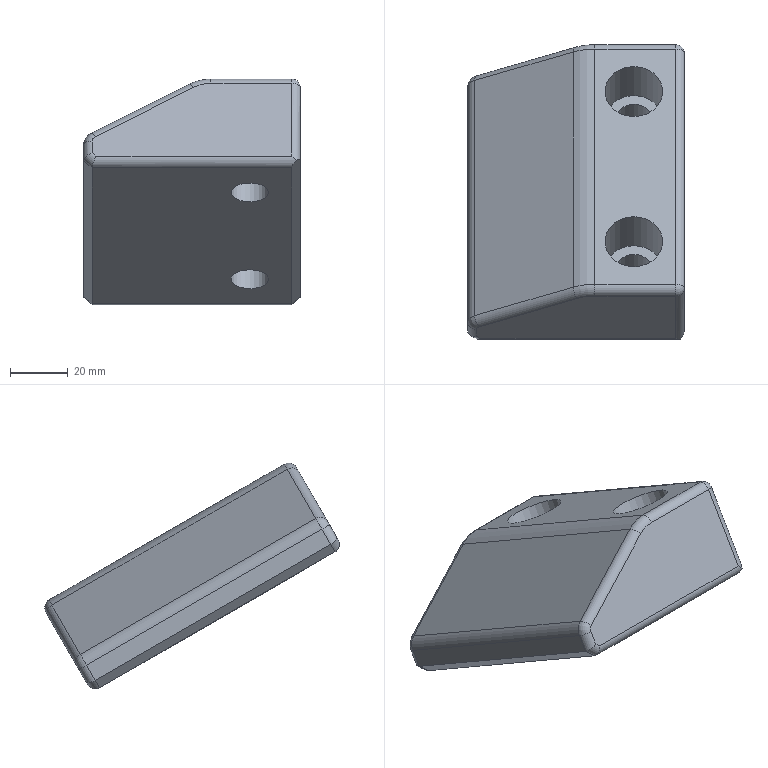Part | NX | features MAIN_BODY 2 | 1 solid | 37 faces | box 75 x 101.906 x 78.115 mm | volume 197655 mm3 | cylinder 20 | plane 11 | torus 4 | sphere 2 | commonest cylinder face diameters 6 x14 13 x2 20 x2 10 x1 30 x1
STEP:
#1=CARTESIAN_POINT('',(342.,445.056,-333.141));
#2=VERTEX_POINT('',#1);
#3=CARTESIAN_POINT('',(342.,363.649,-286.141));
#4=VERTEX_POINT('',#3);
#5=CARTESIAN_POINT('',(342.,361.051,-284.641));
#6=DIRECTION('',(0.,0.866,-0.5));
#7=VECTOR('',#6,1000.);
#8=LINE('',#5,#7);
#9=EDGE_CURVE('',#2,#4,#8,.F.);
#10=ORIENTED_EDGE('',*,*,#9,.F.);
#11=CARTESIAN_POINT('',(342.,442.046,-338.354));
#12=VERTEX_POINT('',#11);
#13=CARTESIAN_POINT('',(342.,445.056,-333.141));
#14=DIRECTION('',(0.,-0.5,-0.866));
#15=VECTOR('',#14,1000.);
#16=LINE('',#13,#15);
#17=EDGE_CURVE('',#12,#2,#16,.F.);
#18=ORIENTED_EDGE('',*,*,#17,.F.);
#19=CARTESIAN_POINT('',(342.,360.64,-291.354));
#20=VERTEX_POINT('',#19);
#21=CARTESIAN_POINT('',(342.,487.945,-364.854));
#22=DIRECTION('',(0.,0.866,-0.5));
#23=VECTOR('',#22,1000.);
#24=LINE('',#21,#23);
#25=EDGE_CURVE('',#20,#12,#24,.T.);
#26=ORIENTED_EDGE('',*,*,#25,.F.);
#27=CARTESIAN_POINT('',(342.,355.14,-300.88));
#28=DIRECTION('',(0.,-0.5,-0.866));
#29=VECTOR('',#28,1000.);
#30=LINE('',#27,#29);
#31=EDGE_CURVE('',#4,#20,#30,.T.);
#32=ORIENTED_EDGE('',*,*,#31,.F.);
#33=EDGE_LOOP('',(#10,#18,#26,#32));
#34=FACE_BOUND('',#33,.T.);
#35=CARTESIAN_POINT('',(342.,692.024,-495.38));
#36=DIRECTION('',(1.,0.,0.));
#37=DIRECTION('',(0.,0.342,-0.9397));
#38=AXIS2_PLACEMENT_3D('',#35,#36,#37);
#39=PLANE('',#38);
#40=ADVANCED_FACE('',(#34),#39,.F.);
#41=CARTESIAN_POINT('',(399.5,400.022,-277.141));
#42=VERTEX_POINT('',#41);
#43=CARTESIAN_POINT('',(399.5,391.362,-272.141));
#44=DIRECTION('',(0.,0.5,0.866));
#45=DIRECTION('',(0.,0.866,-0.5));
#46=AXIS2_PLACEMENT_3D('',#43,#44,#45);
#47=CIRCLE('',#46,10.);
#48=EDGE_CURVE('',#42,#42,#47,.T.);
#49=ORIENTED_EDGE('',*,*,#48,.F.);
#50=EDGE_LOOP('',(#49));
#51=FACE_BOUND('',#50,.T.);
#52=CARTESIAN_POINT('',(399.5,451.984,-307.141));
#53=VERTEX_POINT('',#52);
#54=CARTESIAN_POINT('',(399.5,443.324,-302.141));
#55=DIRECTION('',(0.,0.5,0.866));
#56=DIRECTION('',(0.,0.866,-0.5));
#57=AXIS2_PLACEMENT_3D('',#54,#55,#56);
#58=CIRCLE('',#57,10.);
#59=EDGE_CURVE('',#53,#53,#58,.T.);
#60=ORIENTED_EDGE('',*,*,#59,.F.);
#61=EDGE_LOOP('',(#60));
#62=FACE_BOUND('',#61,.T.);
#63=CARTESIAN_POINT('',(414.,458.046,-310.641));
#64=VERTEX_POINT('',#63);
#65=CARTESIAN_POINT('',(414.,376.64,-263.641));
#66=VERTEX_POINT('',#65);
#67=CARTESIAN_POINT('',(414.,629.519,-409.641));
#68=DIRECTION('',(0.,-0.866,0.5));
#69=VECTOR('',#68,1000.);
#70=LINE('',#67,#69);
#71=EDGE_CURVE('',#64,#66,#70,.T.);
#72=ORIENTED_EDGE('',*,*,#71,.F.);
#73=CARTESIAN_POINT('',(386.019,458.046,-310.641));
#74=VERTEX_POINT('',#73);
#75=CARTESIAN_POINT('',(467.,458.046,-310.641));
#76=DIRECTION('',(1.,0.,0.));
#77=VECTOR('',#76,1000.);
#78=LINE('',#75,#77);
#79=EDGE_CURVE('',#74,#64,#78,.T.);
#80=ORIENTED_EDGE('',*,*,#79,.F.);
#81=CARTESIAN_POINT('',(386.019,376.64,-263.641));
#82=VERTEX_POINT('',#81);
#83=CARTESIAN_POINT('',(386.019,629.519,-409.641));
#84=DIRECTION('',(0.,-0.866,0.5));
#85=VECTOR('',#84,1000.);
#86=LINE('',#83,#85);
#87=EDGE_CURVE('',#82,#74,#86,.F.);
#88=ORIENTED_EDGE('',*,*,#87,.F.);
#89=CARTESIAN_POINT('',(386.019,376.64,-263.641));
#90=DIRECTION('',(-1.,0.,0.));
#91=VECTOR('',#90,1000.);
#92=LINE('',#89,#91);
#93=EDGE_CURVE('',#66,#82,#92,.T.);
#94=ORIENTED_EDGE('',*,*,#93,.F.);
#95=EDGE_LOOP('',(#72,#80,#88,#94));
#96=FACE_BOUND('',#95,.T.);
#97=CARTESIAN_POINT('',(467.,629.519,-409.641));
#98=DIRECTION('',(0.,0.5,0.866));
#99=DIRECTION('',(0.,-0.866,0.5));
#100=AXIS2_PLACEMENT_3D('',#97,#98,#99);
#101=PLANE('',#100);
#102=ADVANCED_FACE('',(#51,#62,#96),#101,.T.);
#103=CARTESIAN_POINT('',(345.,445.265,-338.778));
#104=VERTEX_POINT('',#103);
#105=CARTESIAN_POINT('',(346.243,444.644,-339.854));
#106=VERTEX_POINT('',#105);
#107=CARTESIAN_POINT('',(315.621,459.955,-313.335));
#108=DIRECTION('',(0.7071,-0.3536,-0.6124));
#109=VECTOR('',#108,1000.);
#110=LINE('',#107,#109);
#111=EDGE_CURVE('',#104,#106,#110,.T.);
#112=ORIENTED_EDGE('',*,*,#111,.F.);
#113=CARTESIAN_POINT('',(345.,447.654,-334.641));
#114=VERTEX_POINT('',#113);
#115=CARTESIAN_POINT('',(345.,444.644,-339.854));
#116=DIRECTION('',(0.,-0.5,-0.866));
#117=VECTOR('',#116,1000.);
#118=LINE('',#115,#117);
#119=EDGE_CURVE('',#114,#104,#118,.T.);
#120=ORIENTED_EDGE('',*,*,#119,.F.);
#121=CARTESIAN_POINT('',(346.,448.52,-333.141));
#122=VERTEX_POINT('',#121);
#123=CARTESIAN_POINT('',(347.,447.654,-334.641));
#124=DIRECTION('',(0.,-0.866,0.5));
#125=DIRECTION('',(0.,0.5,0.866));
#126=AXIS2_PLACEMENT_3D('',#123,#124,#125);
#127=CIRCLE('',#126,2.);
#128=EDGE_CURVE('',#122,#114,#127,.T.);
#129=ORIENTED_EDGE('',*,*,#128,.F.);
#130=CARTESIAN_POINT('',(380.019,458.34,-316.131));
#131=VERTEX_POINT('',#130);
#132=CARTESIAN_POINT('',(334.75,445.272,-338.766));
#133=DIRECTION('',(-0.866,-0.25,-0.433));
#134=VECTOR('',#133,1000.);
#135=LINE('',#132,#134);
#136=EDGE_CURVE('',#131,#122,#135,.T.);
#137=ORIENTED_EDGE('',*,*,#136,.F.);
#138=CARTESIAN_POINT('',(386.019,459.144,-314.739));
#139=VERTEX_POINT('',#138);
#140=CARTESIAN_POINT('',(386.019,453.144,-325.131));
#141=DIRECTION('',(0.,-0.866,0.5));
#142=DIRECTION('',(0.,0.5,0.866));
#143=AXIS2_PLACEMENT_3D('',#140,#141,#142);
#144=CIRCLE('',#143,12.);
#145=EDGE_CURVE('',#139,#131,#144,.T.);
#146=ORIENTED_EDGE('',*,*,#145,.F.);
#147=CARTESIAN_POINT('',(414.,459.144,-314.739));
#148=VERTEX_POINT('',#147);
#149=CARTESIAN_POINT('',(317.,459.144,-314.739));
#150=DIRECTION('',(1.,0.,0.));
#151=VECTOR('',#150,1000.);
#152=LINE('',#149,#151);
#153=EDGE_CURVE('',#148,#139,#152,.F.);
#154=ORIENTED_EDGE('',*,*,#153,.F.);
#155=CARTESIAN_POINT('',(414.,445.265,-338.778));
#156=VERTEX_POINT('',#155);
#157=CARTESIAN_POINT('',(414.,460.644,-312.141));
#158=DIRECTION('',(0.,0.5,0.866));
#159=VECTOR('',#158,1000.);
#160=LINE('',#157,#159);
#161=EDGE_CURVE('',#156,#148,#160,.T.);
#162=ORIENTED_EDGE('',*,*,#161,.F.);
#163=CARTESIAN_POINT('',(412.757,444.644,-339.854));
#164=VERTEX_POINT('',#163);
#165=CARTESIAN_POINT('',(380.879,428.705,-367.462));
#166=DIRECTION('',(-0.7071,-0.3536,-0.6124));
#167=VECTOR('',#166,1000.);
#168=LINE('',#165,#167);
#169=EDGE_CURVE('',#164,#156,#168,.F.);
#170=ORIENTED_EDGE('',*,*,#169,.F.);
#171=CARTESIAN_POINT('',(317.,444.644,-339.854));
#172=DIRECTION('',(1.,0.,0.));
#173=VECTOR('',#172,1000.);
#174=LINE('',#171,#173);
#175=EDGE_CURVE('',#106,#164,#174,.T.);
#176=ORIENTED_EDGE('',*,*,#175,.F.);
#177=EDGE_LOOP('',(#112,#120,#129,#137,#146,#154,#162,#170,#176));
#178=FACE_BOUND('',#177,.T.);
#179=CARTESIAN_POINT('',(317.,460.644,-312.141));
#180=DIRECTION('',(0.,0.866,-0.5));
#181=DIRECTION('',(1.,0.,0.));
#182=AXIS2_PLACEMENT_3D('',#179,#180,#181);
#183=PLANE('',#182);
#184=ADVANCED_FACE('',(#178),#183,.T.);
#185=CARTESIAN_POINT('',(414.,358.042,-289.854));
#186=VERTEX_POINT('',#185);
#187=CARTESIAN_POINT('',(346.243,358.042,-289.854));
#188=VERTEX_POINT('',#187);
#189=CARTESIAN_POINT('',(345.,358.042,-289.854));
#190=DIRECTION('',(-1.,0.,0.));
#191=VECTOR('',#190,1000.);
#192=LINE('',#189,#191);
#193=EDGE_CURVE('',#186,#188,#192,.T.);
#194=ORIENTED_EDGE('',*,*,#193,.F.);
#195=CARTESIAN_POINT('',(414.,372.542,-264.739));
#196=VERTEX_POINT('',#195);
#197=CARTESIAN_POINT('',(414.,358.042,-289.854));
#198=DIRECTION('',(0.,0.5,0.866));
#199=VECTOR('',#198,1000.);
#200=LINE('',#197,#199);
#201=EDGE_CURVE('',#196,#186,#200,.F.);
#202=ORIENTED_EDGE('',*,*,#201,.F.);
#203=CARTESIAN_POINT('',(386.019,372.542,-264.739));
#204=VERTEX_POINT('',#203);
#205=CARTESIAN_POINT('',(417.,372.542,-264.739));
#206=DIRECTION('',(-1.,0.,0.));
#207=VECTOR('',#206,1000.);
#208=LINE('',#205,#207);
#209=EDGE_CURVE('',#204,#196,#208,.F.);
#210=ORIENTED_EDGE('',*,*,#209,.F.);
#211=CARTESIAN_POINT('',(380.019,371.738,-266.131));
#212=VERTEX_POINT('',#211);
#213=CARTESIAN_POINT('',(386.019,366.542,-275.131));
#214=DIRECTION('',(0.,-0.866,0.5));
#215=DIRECTION('',(0.,0.5,0.866));
#216=AXIS2_PLACEMENT_3D('',#213,#214,#215);
#217=CIRCLE('',#216,12.);
#218=EDGE_CURVE('',#212,#204,#217,.F.);
#219=ORIENTED_EDGE('',*,*,#218,.F.);
#220=CARTESIAN_POINT('',(346.,361.917,-283.141));
#221=VERTEX_POINT('',#220);
#222=CARTESIAN_POINT('',(380.019,371.738,-266.131));
#223=DIRECTION('',(-0.866,-0.25,-0.433));
#224=VECTOR('',#223,1000.);
#225=LINE('',#222,#224);
#226=EDGE_CURVE('',#221,#212,#225,.F.);
#227=ORIENTED_EDGE('',*,*,#226,.F.);
#228=CARTESIAN_POINT('',(345.,361.051,-284.641));
#229=VERTEX_POINT('',#228);
#230=CARTESIAN_POINT('',(347.,361.051,-284.641));
#231=DIRECTION('',(0.,-0.866,0.5));
#232=DIRECTION('',(0.,0.5,0.866));
#233=AXIS2_PLACEMENT_3D('',#230,#231,#232);
#234=CIRCLE('',#233,2.);
#235=EDGE_CURVE('',#229,#221,#234,.F.);
#236=ORIENTED_EDGE('',*,*,#235,.F.);
#237=CARTESIAN_POINT('',(345.,358.663,-288.778));
#238=VERTEX_POINT('',#237);
#239=CARTESIAN_POINT('',(345.,374.042,-262.141));
#240=DIRECTION('',(0.,-0.5,-0.866));
#241=VECTOR('',#240,1000.);
#242=LINE('',#239,#241);
#243=EDGE_CURVE('',#238,#229,#242,.F.);
#244=ORIENTED_EDGE('',*,*,#243,.F.);
#245=CARTESIAN_POINT('',(344.121,359.102,-288.017));
#246=DIRECTION('',(-0.7071,0.3536,0.6124));
#247=VECTOR('',#246,1000.);
#248=LINE('',#245,#247);
#249=EDGE_CURVE('',#188,#238,#248,.T.);
#250=ORIENTED_EDGE('',*,*,#249,.F.);
#251=EDGE_LOOP('',(#194,#202,#210,#219,#227,#236,#244,#250));
#252=FACE_BOUND('',#251,.T.);
#253=CARTESIAN_POINT('',(317.,374.042,-262.141));
#254=DIRECTION('',(0.,0.866,-0.5));
#255=DIRECTION('',(1.,0.,0.));
#256=AXIS2_PLACEMENT_3D('',#253,#254,#255);
#257=PLANE('',#256);
#258=ADVANCED_FACE('',(#252),#257,.F.);
#259=CARTESIAN_POINT('',(399.5,379.491,-305.702));
#260=VERTEX_POINT('',#259);
#261=CARTESIAN_POINT('',(399.5,373.862,-302.452));
#262=DIRECTION('',(0.,0.5,0.866));
#263=DIRECTION('',(0.,0.866,-0.5));
#264=AXIS2_PLACEMENT_3D('',#261,#262,#263);
#265=CIRCLE('',#264,6.5);
#266=EDGE_CURVE('',#260,#260,#265,.T.);
#267=ORIENTED_EDGE('',*,*,#266,.T.);
#268=EDGE_LOOP('',(#267));
#269=FACE_BOUND('',#268,.T.);
#270=CARTESIAN_POINT('',(399.5,431.453,-335.702));
#271=VERTEX_POINT('',#270);
#272=CARTESIAN_POINT('',(399.5,425.824,-332.452));
#273=DIRECTION('',(0.,0.5,0.866));
#274=DIRECTION('',(0.,0.866,-0.5));
#275=AXIS2_PLACEMENT_3D('',#272,#273,#274);
#276=CIRCLE('',#275,6.5);
#277=EDGE_CURVE('',#271,#271,#276,.T.);
#278=ORIENTED_EDGE('',*,*,#277,.T.);
#279=EDGE_LOOP('',(#278));
#280=FACE_BOUND('',#279,.T.);
#281=CARTESIAN_POINT('',(414.,440.546,-340.952));
#282=VERTEX_POINT('',#281);
#283=CARTESIAN_POINT('',(414.,359.14,-293.952));
#284=VERTEX_POINT('',#283);
#285=CARTESIAN_POINT('',(414.,612.019,-439.952));
#286=DIRECTION('',(0.,-0.866,0.5));
#287=VECTOR('',#286,1000.);
#288=LINE('',#285,#287);
#289=EDGE_CURVE('',#282,#284,#288,.T.);
#290=ORIENTED_EDGE('',*,*,#289,.T.);
#291=CARTESIAN_POINT('',(345.,359.14,-293.952));
#292=VERTEX_POINT('',#291);
#293=CARTESIAN_POINT('',(414.,359.14,-293.952));
#294=DIRECTION('',(-1.,0.,0.));
#295=VECTOR('',#294,1000.);
#296=LINE('',#293,#295);
#297=EDGE_CURVE('',#292,#284,#296,.F.);
#298=ORIENTED_EDGE('',*,*,#297,.F.);
#299=CARTESIAN_POINT('',(345.,440.546,-340.952));
#300=VERTEX_POINT('',#299);
#301=CARTESIAN_POINT('',(345.,356.542,-292.452));
#302=DIRECTION('',(0.,-0.866,0.5));
#303=VECTOR('',#302,1000.);
#304=LINE('',#301,#303);
#305=EDGE_CURVE('',#300,#292,#304,.T.);
#306=ORIENTED_EDGE('',*,*,#305,.F.);
#307=CARTESIAN_POINT('',(317.,440.546,-340.952));
#308=DIRECTION('',(1.,0.,0.));
#309=VECTOR('',#308,1000.);
#310=LINE('',#307,#309);
#311=EDGE_CURVE('',#282,#300,#310,.F.);
#312=ORIENTED_EDGE('',*,*,#311,.F.);
#313=EDGE_LOOP('',(#290,#298,#306,#312));
#314=FACE_BOUND('',#313,.T.);
#315=CARTESIAN_POINT('',(317.,612.019,-439.952));
#316=DIRECTION('',(0.,-0.5,-0.866));
#317=DIRECTION('',(-1.,0.,0.));
#318=AXIS2_PLACEMENT_3D('',#315,#316,#317);
#319=PLANE('',#318);
#320=ADVANCED_FACE('',(#269,#280,#314),#319,.T.);
#321=CARTESIAN_POINT('',(417.,375.14,-266.239));
#322=VERTEX_POINT('',#321);
#323=CARTESIAN_POINT('',(417.,456.546,-313.239));
#324=VERTEX_POINT('',#323);
#325=CARTESIAN_POINT('',(417.,628.019,-412.239));
#326=DIRECTION('',(0.,-0.866,0.5));
#327=VECTOR('',#326,1000.);
#328=LINE('',#325,#327);
#329=EDGE_CURVE('',#322,#324,#328,.F.);
#330=ORIENTED_EDGE('',*,*,#329,.F.);
#331=CARTESIAN_POINT('',(417.,360.64,-291.354));
#332=VERTEX_POINT('',#331);
#333=CARTESIAN_POINT('',(417.,376.64,-263.641));
#334=DIRECTION('',(0.,0.5,0.866));
#335=VECTOR('',#334,1000.);
#336=LINE('',#333,#335);
#337=EDGE_CURVE('',#332,#322,#336,.T.);
#338=ORIENTED_EDGE('',*,*,#337,.F.);
#339=CARTESIAN_POINT('',(417.,442.046,-338.354));
#340=VERTEX_POINT('',#339);
#341=CARTESIAN_POINT('',(417.,613.519,-437.354));
#342=DIRECTION('',(0.,-0.866,0.5));
#343=VECTOR('',#342,1000.);
#344=LINE('',#341,#343);
#345=EDGE_CURVE('',#340,#332,#344,.T.);
#346=ORIENTED_EDGE('',*,*,#345,.F.);
#347=CARTESIAN_POINT('',(417.,435.546,-349.612));
#348=DIRECTION('',(0.,0.5,0.866));
#349=VECTOR('',#348,1000.);
#350=LINE('',#347,#349);
#351=EDGE_CURVE('',#324,#340,#350,.F.);
#352=ORIENTED_EDGE('',*,*,#351,.F.);
#353=EDGE_LOOP('',(#330,#338,#346,#352));
#354=FACE_BOUND('',#353,.T.);
#355=CARTESIAN_POINT('',(417.,607.019,-448.612));
#356=DIRECTION('',(1.,0.,0.));
#357=DIRECTION('',(0.,-0.866,0.5));
#358=AXIS2_PLACEMENT_3D('',#355,#356,#357);
#359=PLANE('',#358);
#360=ADVANCED_FACE('',(#354),#359,.T.);
#361=CARTESIAN_POINT('',(378.519,457.041,-312.381));
#362=VERTEX_POINT('',#361);
#363=CARTESIAN_POINT('',(378.519,375.635,-265.381));
#364=VERTEX_POINT('',#363);
#365=CARTESIAN_POINT('',(378.519,502.941,-338.881));
#366=DIRECTION('',(0.,-0.866,0.5));
#367=VECTOR('',#366,1000.);
#368=LINE('',#365,#367);
#369=EDGE_CURVE('',#362,#364,#368,.T.);
#370=ORIENTED_EDGE('',*,*,#369,.F.);
#371=CARTESIAN_POINT('',(344.5,447.221,-329.391));
#372=VERTEX_POINT('',#371);
#373=CARTESIAN_POINT('',(382.,458.046,-310.641));
#374=DIRECTION('',(-0.866,-0.25,-0.433));
#375=VECTOR('',#374,1000.);
#376=LINE('',#373,#375);
#377=EDGE_CURVE('',#372,#362,#376,.F.);
#378=ORIENTED_EDGE('',*,*,#377,.F.);
#379=CARTESIAN_POINT('',(344.5,365.814,-282.391));
#380=VERTEX_POINT('',#379);
#381=CARTESIAN_POINT('',(344.5,493.12,-355.891));
#382=DIRECTION('',(0.,0.866,-0.5));
#383=VECTOR('',#382,1000.);
#384=LINE('',#381,#383);
#385=EDGE_CURVE('',#380,#372,#384,.T.);
#386=ORIENTED_EDGE('',*,*,#385,.F.);
#387=CARTESIAN_POINT('',(344.5,365.814,-282.391));
#388=DIRECTION('',(-0.866,-0.25,-0.433));
#389=VECTOR('',#388,1000.);
#390=LINE('',#387,#389);
#391=EDGE_CURVE('',#364,#380,#390,.T.);
#392=ORIENTED_EDGE('',*,*,#391,.F.);
#393=EDGE_LOOP('',(#370,#378,#386,#392));
#394=FACE_BOUND('',#393,.T.);
#395=CARTESIAN_POINT('',(382.,503.945,-337.141));
#396=DIRECTION('',(-0.5,0.433,0.75));
#397=DIRECTION('',(0.,-0.866,0.5));
#398=AXIS2_PLACEMENT_3D('',#395,#396,#397);
#399=PLANE('',#398);
#400=ADVANCED_FACE('',(#394),#399,.T.);
#401=CARTESIAN_POINT('',(399.5,438.953,-322.712));
#402=VERTEX_POINT('',#401);
#403=CARTESIAN_POINT('',(399.5,433.324,-319.462));
#404=DIRECTION('',(0.,0.5,0.866));
#405=DIRECTION('',(0.,0.866,-0.5));
#406=AXIS2_PLACEMENT_3D('',#403,#404,#405);
#407=CIRCLE('',#406,6.5);
#408=EDGE_CURVE('',#402,#402,#407,.T.);
#409=ORIENTED_EDGE('',*,*,#408,.F.);
#410=EDGE_LOOP('',(#409));
#411=FACE_BOUND('',#410,.T.);
#412=CARTESIAN_POINT('',(399.5,441.984,-324.462));
#413=VERTEX_POINT('',#412);
#414=CARTESIAN_POINT('',(399.5,433.324,-319.462));
#415=DIRECTION('',(0.,0.5,0.866));
#416=DIRECTION('',(0.,0.866,-0.5));
#417=AXIS2_PLACEMENT_3D('',#414,#415,#416);
#418=CIRCLE('',#417,10.);
#419=EDGE_CURVE('',#413,#413,#418,.T.);
#420=ORIENTED_EDGE('',*,*,#419,.T.);
#421=EDGE_LOOP('',(#420));
#422=FACE_BOUND('',#421,.T.);
#423=CARTESIAN_POINT('',(399.5,433.324,-319.462));
#424=DIRECTION('',(0.,-0.5,-0.866));
#425=DIRECTION('',(0.,0.866,-0.5));
#426=AXIS2_PLACEMENT_3D('',#423,#424,#425);
#427=PLANE('',#426);
#428=ADVANCED_FACE('',(#411,#422),#427,.F.);
#429=ORIENTED_EDGE('',*,*,#419,.F.);
#430=EDGE_LOOP('',(#429));
#431=FACE_BOUND('',#430,.T.);
#432=ORIENTED_EDGE('',*,*,#59,.T.);
#433=EDGE_LOOP('',(#432));
#434=FACE_BOUND('',#433,.T.);
#435=CARTESIAN_POINT('',(399.5,443.324,-302.141));
#436=DIRECTION('',(0.,-0.5,-0.866));
#437=DIRECTION('',(0.,0.866,-0.5));
#438=AXIS2_PLACEMENT_3D('',#435,#436,#437);
#439=CYLINDRICAL_SURFACE('',#438,10.);
#440=ADVANCED_FACE('',(#431,#434),#439,.F.);
#441=CARTESIAN_POINT('',(399.5,386.991,-292.712));
#442=VERTEX_POINT('',#441);
#443=CARTESIAN_POINT('',(399.5,381.362,-289.462));
#444=DIRECTION('',(0.,0.5,0.866));
#445=DIRECTION('',(0.,0.866,-0.5));
#446=AXIS2_PLACEMENT_3D('',#443,#444,#445);
#447=CIRCLE('',#446,6.5);
#448=EDGE_CURVE('',#442,#442,#447,.T.);
#449=ORIENTED_EDGE('',*,*,#448,.F.);
#450=EDGE_LOOP('',(#449));
#451=FACE_BOUND('',#450,.T.);
#452=CARTESIAN_POINT('',(399.5,390.022,-294.462));
#453=VERTEX_POINT('',#452);
#454=CARTESIAN_POINT('',(399.5,381.362,-289.462));
#455=DIRECTION('',(0.,0.5,0.866));
#456=DIRECTION('',(0.,0.866,-0.5));
#457=AXIS2_PLACEMENT_3D('',#454,#455,#456);
#458=CIRCLE('',#457,10.);
#459=EDGE_CURVE('',#453,#453,#458,.T.);
#460=ORIENTED_EDGE('',*,*,#459,.T.);
#461=EDGE_LOOP('',(#460));
#462=FACE_BOUND('',#461,.T.);
#463=CARTESIAN_POINT('',(399.5,381.362,-289.462));
#464=DIRECTION('',(0.,-0.5,-0.866));
#465=DIRECTION('',(0.,0.866,-0.5));
#466=AXIS2_PLACEMENT_3D('',#463,#464,#465);
#467=PLANE('',#466);
#468=ADVANCED_FACE('',(#451,#462),#467,.F.);
#469=ORIENTED_EDGE('',*,*,#459,.F.);
#470=EDGE_LOOP('',(#469));
#471=FACE_BOUND('',#470,.T.);
#472=ORIENTED_EDGE('',*,*,#48,.T.);
#473=EDGE_LOOP('',(#472));
#474=FACE_BOUND('',#473,.T.);
#475=CARTESIAN_POINT('',(399.5,391.362,-272.141));
#476=DIRECTION('',(0.,-0.5,-0.866));
#477=DIRECTION('',(0.,0.866,-0.5));
#478=AXIS2_PLACEMENT_3D('',#475,#476,#477);
#479=CYLINDRICAL_SURFACE('',#478,10.);
#480=ADVANCED_FACE('',(#471,#474),#479,.F.);
#481=ORIENTED_EDGE('',*,*,#277,.F.);
#482=EDGE_LOOP('',(#481));
#483=FACE_BOUND('',#482,.T.);
#484=ORIENTED_EDGE('',*,*,#408,.T.);
#485=EDGE_LOOP('',(#484));
#486=FACE_BOUND('',#485,.T.);
#487=CARTESIAN_POINT('',(399.5,433.324,-319.462));
#488=DIRECTION('',(0.,-0.5,-0.866));
#489=DIRECTION('',(0.,0.866,-0.5));
#490=AXIS2_PLACEMENT_3D('',#487,#488,#489);
#491=CYLINDRICAL_SURFACE('',#490,6.5);
#492=ADVANCED_FACE('',(#483,#486),#491,.F.);
#493=ORIENTED_EDGE('',*,*,#266,.F.);
#494=EDGE_LOOP('',(#493));
#495=FACE_BOUND('',#494,.T.);
#496=ORIENTED_EDGE('',*,*,#448,.T.);
#497=EDGE_LOOP('',(#496));
#498=FACE_BOUND('',#497,.T.);
#499=CARTESIAN_POINT('',(399.5,381.362,-289.462));
#500=DIRECTION('',(0.,-0.5,-0.866));
#501=DIRECTION('',(0.,0.866,-0.5));
#502=AXIS2_PLACEMENT_3D('',#499,#500,#501);
#503=CYLINDRICAL_SURFACE('',#502,6.5);
#504=ADVANCED_FACE('',(#495,#498),#503,.F.);
#505=ORIENTED_EDGE('',*,*,#345,.T.);
#506=CARTESIAN_POINT('',(415.5,357.64,-291.354));
#507=VERTEX_POINT('',#506);
#508=CARTESIAN_POINT('',(414.,359.14,-293.952));
#509=DIRECTION('',(0.7071,-0.3536,-0.6124));
#510=DIRECTION('',(-0.7071,-0.3536,-0.6124));
#511=AXIS2_PLACEMENT_3D('',#508,#509,#510);
#512=ELLIPSE('',#511,4.243,3.);
#513=EDGE_CURVE('',#507,#332,#512,.F.);
#514=ORIENTED_EDGE('',*,*,#513,.F.);
#515=CARTESIAN_POINT('',(417.,360.64,-291.354));
#516=DIRECTION('',(0.7071,-0.3536,-0.6124));
#517=DIRECTION('',(0.7071,0.3536,0.6124));
#518=AXIS2_PLACEMENT_3D('',#515,#516,#517);
#519=ELLIPSE('',#518,4.243,3.);
#520=EDGE_CURVE('',#284,#507,#519,.F.);
#521=ORIENTED_EDGE('',*,*,#520,.F.);
#522=ORIENTED_EDGE('',*,*,#289,.F.);
#523=CARTESIAN_POINT('',(414.,440.546,-340.952));
#524=DIRECTION('',(0.7071,0.3536,0.6124));
#525=VECTOR('',#524,1000.);
#526=LINE('',#523,#525);
#527=EDGE_CURVE('',#340,#282,#526,.F.);
#528=ORIENTED_EDGE('',*,*,#527,.F.);
#529=EDGE_LOOP('',(#505,#514,#521,#522,#528));
#530=FACE_BOUND('',#529,.T.);
#531=CARTESIAN_POINT('',(414.,612.019,-439.952));
#532=DIRECTION('',(-0.7071,0.3536,0.6124));
#533=DIRECTION('',(0.6715,0.607,0.425));
#534=AXIS2_PLACEMENT_3D('',#531,#532,#533);
#535=PLANE('',#534);
#536=ADVANCED_FACE('',(#530),#535,.F.);
#537=ORIENTED_EDGE('',*,*,#25,.T.);
#538=CARTESIAN_POINT('',(342.,442.046,-338.354));
#539=DIRECTION('',(0.7071,-0.3536,-0.6124));
#540=VECTOR('',#539,1000.);
#541=LINE('',#538,#540);
#542=EDGE_CURVE('',#300,#12,#541,.F.);
#543=ORIENTED_EDGE('',*,*,#542,.F.);
#544=ORIENTED_EDGE('',*,*,#305,.T.);
#545=CARTESIAN_POINT('',(345.,359.14,-293.952));
#546=DIRECTION('',(-0.7071,0.3536,0.6124));
#547=VECTOR('',#546,1000.);
#548=LINE('',#545,#547);
#549=EDGE_CURVE('',#20,#292,#548,.F.);
#550=ORIENTED_EDGE('',*,*,#549,.F.);
#551=EDGE_LOOP('',(#537,#543,#544,#550));
#552=FACE_BOUND('',#551,.T.);
#553=CARTESIAN_POINT('',(342.,697.524,-485.854));
#554=DIRECTION('',(-0.7071,-0.3536,-0.6124));
#555=DIRECTION('',(-0.6715,0.607,0.425));
#556=AXIS2_PLACEMENT_3D('',#553,#554,#555);
#557=PLANE('',#556);
#558=ADVANCED_FACE('',(#552),#557,.T.);
#559=ORIENTED_EDGE('',*,*,#385,.T.);
#560=CARTESIAN_POINT('',(347.,445.056,-333.141));
#561=DIRECTION('',(0.,-0.866,0.5));
#562=DIRECTION('',(0.,0.5,0.866));
#563=AXIS2_PLACEMENT_3D('',#560,#561,#562);
#564=CIRCLE('',#563,5.);
#565=EDGE_CURVE('',#2,#372,#564,.F.);
#566=ORIENTED_EDGE('',*,*,#565,.F.);
#567=ORIENTED_EDGE('',*,*,#9,.T.);
#568=CARTESIAN_POINT('',(347.,363.649,-286.141));
#569=DIRECTION('',(0.,-0.866,0.5));
#570=DIRECTION('',(0.,0.5,0.866));
#571=AXIS2_PLACEMENT_3D('',#568,#569,#570);
#572=CIRCLE('',#571,5.);
#573=EDGE_CURVE('',#380,#4,#572,.T.);
#574=ORIENTED_EDGE('',*,*,#573,.F.);
#575=EDGE_LOOP('',(#559,#566,#567,#574));
#576=FACE_BOUND('',#575,.T.);
#577=CARTESIAN_POINT('',(347.,490.955,-359.641));
#578=DIRECTION('',(0.,-0.866,0.5));
#579=DIRECTION('',(0.,-0.5,-0.866));
#580=AXIS2_PLACEMENT_3D('',#577,#578,#579);
#581=CYLINDRICAL_SURFACE('',#580,5.);
#582=ADVANCED_FACE('',(#576),#581,.T.);
#583=ORIENTED_EDGE('',*,*,#87,.T.);
#584=CARTESIAN_POINT('',(386.019,450.546,-323.631));
#585=DIRECTION('',(0.,-0.866,0.5));
#586=DIRECTION('',(0.,0.5,0.866));
#587=AXIS2_PLACEMENT_3D('',#584,#585,#586);
#588=CIRCLE('',#587,15.);
#589=EDGE_CURVE('',#362,#74,#588,.F.);
#590=ORIENTED_EDGE('',*,*,#589,.F.);
#591=ORIENTED_EDGE('',*,*,#369,.T.);
#592=CARTESIAN_POINT('',(386.019,369.14,-276.631));
#593=DIRECTION('',(0.,-0.866,0.5));
#594=DIRECTION('',(0.,0.5,0.866));
#595=AXIS2_PLACEMENT_3D('',#592,#593,#594);
#596=CIRCLE('',#595,15.);
#597=EDGE_CURVE('',#82,#364,#596,.T.);
#598=ORIENTED_EDGE('',*,*,#597,.F.);
#599=EDGE_LOOP('',(#583,#590,#591,#598));
#600=FACE_BOUND('',#599,.T.);
#601=CARTESIAN_POINT('',(386.019,496.445,-350.131));
#602=DIRECTION('',(0.,-0.866,0.5));
#603=DIRECTION('',(0.,-0.5,-0.866));
#604=AXIS2_PLACEMENT_3D('',#601,#602,#603);
#605=CYLINDRICAL_SURFACE('',#604,15.);
#606=ADVANCED_FACE('',(#600),#605,.T.);
#607=CARTESIAN_POINT('',(345.,445.056,-333.141));
#608=DIRECTION('',(0.,-0.5,-0.866));
#609=DIRECTION('',(0.,-0.866,0.5));
#610=AXIS2_PLACEMENT_3D('',#607,#608,#609);
#611=CIRCLE('',#610,3.);
#612=EDGE_CURVE('',#2,#114,#611,.T.);
#613=ORIENTED_EDGE('',*,*,#612,.T.);
#614=ORIENTED_EDGE('',*,*,#119,.T.);
#615=CARTESIAN_POINT('',(345.,442.667,-337.278));
#616=DIRECTION('',(0.3827,-0.4619,-0.8001));
#617=DIRECTION('',(0.9239,0.1913,0.3314));
#618=AXIS2_PLACEMENT_3D('',#615,#616,#617);
#619=ELLIPSE('',#618,3.247,3.);
#620=EDGE_CURVE('',#104,#12,#619,.F.);
#621=ORIENTED_EDGE('',*,*,#620,.T.);
#622=ORIENTED_EDGE('',*,*,#17,.T.);
#623=EDGE_LOOP('',(#613,#614,#621,#622));
#624=FACE_BOUND('',#623,.T.);
#625=CARTESIAN_POINT('',(345.,458.046,-310.641));
#626=DIRECTION('',(0.,0.5,0.866));
#627=DIRECTION('',(0.,-0.866,0.5));
#628=AXIS2_PLACEMENT_3D('',#625,#626,#627);
#629=CYLINDRICAL_SURFACE('',#628,3.);
#630=ADVANCED_FACE('',(#624),#629,.T.);
#631=ORIENTED_EDGE('',*,*,#620,.F.);
#632=ORIENTED_EDGE('',*,*,#111,.T.);
#633=CARTESIAN_POINT('',(346.243,442.046,-338.354));
#634=DIRECTION('',(-0.9239,0.1913,0.3314));
#635=DIRECTION('',(0.3827,0.4619,0.8001));
#636=AXIS2_PLACEMENT_3D('',#633,#634,#635);
#637=ELLIPSE('',#636,3.247,3.);
#638=EDGE_CURVE('',#106,#300,#637,.T.);
#639=ORIENTED_EDGE('',*,*,#638,.T.);
#640=ORIENTED_EDGE('',*,*,#542,.T.);
#641=EDGE_LOOP('',(#631,#632,#639,#640));
#642=FACE_BOUND('',#641,.T.);
#643=CARTESIAN_POINT('',(315.621,457.357,-311.835));
#644=DIRECTION('',(0.7071,-0.3536,-0.6124));
#645=DIRECTION('',(-0.6715,-0.607,-0.425));
#646=AXIS2_PLACEMENT_3D('',#643,#644,#645);
#647=CYLINDRICAL_SURFACE('',#646,3.);
#648=ADVANCED_FACE('',(#642),#647,.T.);
#649=ORIENTED_EDGE('',*,*,#612,.F.);
#650=ORIENTED_EDGE('',*,*,#565,.T.);
#651=CARTESIAN_POINT('',(346.,445.922,-331.641));
#652=DIRECTION('',(-0.866,-0.25,-0.433));
#653=DIRECTION('',(0.4636,-0.7258,-0.5082));
#654=AXIS2_PLACEMENT_3D('',#651,#652,#653);
#655=CIRCLE('',#654,3.);
#656=EDGE_CURVE('',#372,#122,#655,.T.);
#657=ORIENTED_EDGE('',*,*,#656,.T.);
#658=ORIENTED_EDGE('',*,*,#128,.T.);
#659=EDGE_LOOP('',(#649,#650,#657,#658));
#660=FACE_BOUND('',#659,.T.);
#661=CARTESIAN_POINT('',(347.,445.056,-333.141));
#662=DIRECTION('',(0.,0.866,-0.5));
#663=DIRECTION('',(0.,0.5,0.866));
#664=AXIS2_PLACEMENT_3D('',#661,#662,#663);
#665=DEGENERATE_TOROIDAL_SURFACE('',#664,2.,3.,.T.);
#666=ADVANCED_FACE('',(#660),#665,.T.);
#667=ORIENTED_EDGE('',*,*,#638,.F.);
#668=ORIENTED_EDGE('',*,*,#175,.T.);
#669=CARTESIAN_POINT('',(412.757,442.046,-338.354));
#670=DIRECTION('',(-0.9239,-0.1913,-0.3314));
#671=DIRECTION('',(0.3827,-0.4619,-0.8001));
#672=AXIS2_PLACEMENT_3D('',#669,#670,#671);
#673=ELLIPSE('',#672,3.247,3.);
#674=EDGE_CURVE('',#164,#282,#673,.T.);
#675=ORIENTED_EDGE('',*,*,#674,.T.);
#676=ORIENTED_EDGE('',*,*,#311,.T.);
#677=EDGE_LOOP('',(#667,#668,#675,#676));
#678=FACE_BOUND('',#677,.T.);
#679=CARTESIAN_POINT('',(317.,442.046,-338.354));
#680=DIRECTION('',(1.,0.,0.));
#681=DIRECTION('',(0.,-0.5736,0.8192));
#682=AXIS2_PLACEMENT_3D('',#679,#680,#681);
#683=CYLINDRICAL_SURFACE('',#682,3.);
#684=ADVANCED_FACE('',(#678),#683,.T.);
#685=ORIENTED_EDGE('',*,*,#656,.F.);
#686=ORIENTED_EDGE('',*,*,#377,.T.);
#687=CARTESIAN_POINT('',(380.019,455.742,-314.631));
#688=DIRECTION('',(-0.866,-0.25,-0.433));
#689=DIRECTION('',(0.4636,-0.7258,-0.5082));
#690=AXIS2_PLACEMENT_3D('',#687,#688,#689);
#691=CIRCLE('',#690,3.);
#692=EDGE_CURVE('',#362,#131,#691,.T.);
#693=ORIENTED_EDGE('',*,*,#692,.T.);
#694=ORIENTED_EDGE('',*,*,#136,.T.);
#695=EDGE_LOOP('',(#685,#686,#693,#694));
#696=FACE_BOUND('',#695,.T.);
#697=CARTESIAN_POINT('',(334.75,442.674,-337.266));
#698=DIRECTION('',(-0.866,-0.25,-0.433));
#699=DIRECTION('',(-0.4636,0.7258,0.5082));
#700=AXIS2_PLACEMENT_3D('',#697,#698,#699);
#701=CYLINDRICAL_SURFACE('',#700,3.);
#702=ADVANCED_FACE('',(#696),#701,.T.);
#703=ORIENTED_EDGE('',*,*,#674,.F.);
#704=ORIENTED_EDGE('',*,*,#169,.T.);
#705=CARTESIAN_POINT('',(414.,442.667,-337.278));
#706=DIRECTION('',(-0.3827,-0.4619,-0.8001));
#707=DIRECTION('',(-0.9239,0.1913,0.3314));
#708=AXIS2_PLACEMENT_3D('',#705,#706,#707);
#709=ELLIPSE('',#708,3.247,3.);
#710=EDGE_CURVE('',#156,#340,#709,.T.);
#711=ORIENTED_EDGE('',*,*,#710,.T.);
#712=ORIENTED_EDGE('',*,*,#527,.T.);
#713=EDGE_LOOP('',(#703,#704,#711,#712));
#714=FACE_BOUND('',#713,.T.);
#715=CARTESIAN_POINT('',(380.879,426.107,-365.962));
#716=DIRECTION('',(-0.7071,-0.3536,-0.6124));
#717=DIRECTION('',(-0.6715,0.607,0.425));
#718=AXIS2_PLACEMENT_3D('',#715,#716,#717);
#719=CYLINDRICAL_SURFACE('',#718,3.);
#720=ADVANCED_FACE('',(#714),#719,.T.);
#721=ORIENTED_EDGE('',*,*,#692,.F.);
#722=ORIENTED_EDGE('',*,*,#589,.T.);
#723=CARTESIAN_POINT('',(386.019,456.546,-313.239));
#724=DIRECTION('',(-1.,0.,0.));
#725=DIRECTION('',(0.,-0.8192,-0.5736));
#726=AXIS2_PLACEMENT_3D('',#723,#724,#725);
#727=CIRCLE('',#726,3.);
#728=EDGE_CURVE('',#74,#139,#727,.T.);
#729=ORIENTED_EDGE('',*,*,#728,.T.);
#730=ORIENTED_EDGE('',*,*,#145,.T.);
#731=EDGE_LOOP('',(#721,#722,#729,#730));
#732=FACE_BOUND('',#731,.T.);
#733=CARTESIAN_POINT('',(386.019,450.546,-323.631));
#734=DIRECTION('',(0.,0.866,-0.5));
#735=DIRECTION('',(0.,0.5,0.866));
#736=AXIS2_PLACEMENT_3D('',#733,#734,#735);
#737=TOROIDAL_SURFACE('',#736,12.,3.);
#738=ADVANCED_FACE('',(#732),#737,.T.);
#739=ORIENTED_EDGE('',*,*,#710,.F.);
#740=ORIENTED_EDGE('',*,*,#161,.T.);
#741=CARTESIAN_POINT('',(414.,456.546,-313.239));
#742=DIRECTION('',(0.,-0.5,-0.866));
#743=DIRECTION('',(0.,-0.866,0.5));
#744=AXIS2_PLACEMENT_3D('',#741,#742,#743);
#745=CIRCLE('',#744,3.);
#746=EDGE_CURVE('',#148,#324,#745,.T.);
#747=ORIENTED_EDGE('',*,*,#746,.T.);
#748=ORIENTED_EDGE('',*,*,#351,.T.);
#749=EDGE_LOOP('',(#739,#740,#747,#748));
#750=FACE_BOUND('',#749,.T.);
#751=CARTESIAN_POINT('',(414.,458.046,-310.641));
#752=DIRECTION('',(0.,0.5,0.866));
#753=DIRECTION('',(0.,-0.866,0.5));
#754=AXIS2_PLACEMENT_3D('',#751,#752,#753);
#755=CYLINDRICAL_SURFACE('',#754,3.);
#756=ADVANCED_FACE('',(#750),#755,.T.);
#757=ORIENTED_EDGE('',*,*,#728,.F.);
#758=ORIENTED_EDGE('',*,*,#79,.T.);
#759=CARTESIAN_POINT('',(414.,456.546,-313.239));
#760=DIRECTION('',(-1.,0.,0.));
#761=DIRECTION('',(0.,-0.8192,-0.5736));
#762=AXIS2_PLACEMENT_3D('',#759,#760,#761);
#763=CIRCLE('',#762,3.);
#764=EDGE_CURVE('',#64,#148,#763,.T.);
#765=ORIENTED_EDGE('',*,*,#764,.T.);
#766=ORIENTED_EDGE('',*,*,#153,.T.);
#767=EDGE_LOOP('',(#757,#758,#765,#766));
#768=FACE_BOUND('',#767,.T.);
#769=CARTESIAN_POINT('',(467.,456.546,-313.239));
#770=DIRECTION('',(1.,0.,0.));
#771=DIRECTION('',(0.,-0.5736,0.8192));
#772=AXIS2_PLACEMENT_3D('',#769,#770,#771);
#773=CYLINDRICAL_SURFACE('',#772,3.);
#774=ADVANCED_FACE('',(#768),#773,.T.);
#775=ORIENTED_EDGE('',*,*,#764,.F.);
#776=CARTESIAN_POINT('',(414.,456.546,-313.239));
#777=DIRECTION('',(0.,-0.866,0.5));
#778=DIRECTION('',(0.,0.5,0.866));
#779=AXIS2_PLACEMENT_3D('',#776,#777,#778);
#780=CIRCLE('',#779,3.);
#781=EDGE_CURVE('',#64,#324,#780,.F.);
#782=ORIENTED_EDGE('',*,*,#781,.T.);
#783=ORIENTED_EDGE('',*,*,#746,.F.);
#784=EDGE_LOOP('',(#775,#782,#783));
#785=FACE_BOUND('',#784,.T.);
#786=CARTESIAN_POINT('',(414.,456.546,-313.239));
#787=DIRECTION('',(0.,0.8192,0.5736));
#788=DIRECTION('',(0.,-0.5736,0.8192));
#789=AXIS2_PLACEMENT_3D('',#786,#787,#788);
#790=SPHERICAL_SURFACE('',#789,3.);
#791=ADVANCED_FACE('',(#785),#790,.T.);
#792=ORIENTED_EDGE('',*,*,#781,.F.);
#793=ORIENTED_EDGE('',*,*,#71,.T.);
#794=CARTESIAN_POINT('',(414.,375.14,-266.239));
#795=DIRECTION('',(0.,0.866,-0.5));
#796=DIRECTION('',(0.,-0.5,-0.866));
#797=AXIS2_PLACEMENT_3D('',#794,#795,#796);
#798=CIRCLE('',#797,3.);
#799=EDGE_CURVE('',#66,#322,#798,.T.);
#800=ORIENTED_EDGE('',*,*,#799,.T.);
#801=ORIENTED_EDGE('',*,*,#329,.T.);
#802=EDGE_LOOP('',(#792,#793,#800,#801));
#803=FACE_BOUND('',#802,.T.);
#804=CARTESIAN_POINT('',(414.,628.019,-412.239));
#805=DIRECTION('',(0.,-0.866,0.5));
#806=DIRECTION('',(0.,-0.5,-0.866));
#807=AXIS2_PLACEMENT_3D('',#804,#805,#806);
#808=CYLINDRICAL_SURFACE('',#807,3.);
#809=ADVANCED_FACE('',(#803),#808,.T.);
#810=CARTESIAN_POINT('',(414.,375.14,-266.239));
#811=DIRECTION('',(-1.,0.,0.));
#812=DIRECTION('',(0.,-0.8192,-0.5736));
#813=AXIS2_PLACEMENT_3D('',#810,#811,#812);
#814=CIRCLE('',#813,3.);
#815=EDGE_CURVE('',#196,#66,#814,.T.);
#816=ORIENTED_EDGE('',*,*,#815,.T.);
#817=ORIENTED_EDGE('',*,*,#93,.T.);
#818=CARTESIAN_POINT('',(386.019,375.14,-266.239));
#819=DIRECTION('',(1.,0.,0.));
#820=DIRECTION('',(0.,0.8192,0.5736));
#821=AXIS2_PLACEMENT_3D('',#818,#819,#820);
#822=CIRCLE('',#821,3.);
#823=EDGE_CURVE('',#82,#204,#822,.T.);
#824=ORIENTED_EDGE('',*,*,#823,.T.);
#825=ORIENTED_EDGE('',*,*,#209,.T.);
#826=EDGE_LOOP('',(#816,#817,#824,#825));
#827=FACE_BOUND('',#826,.T.);
#828=CARTESIAN_POINT('',(467.,375.14,-266.239));
#829=DIRECTION('',(1.,0.,0.));
#830=DIRECTION('',(0.,-0.5736,0.8192));
#831=AXIS2_PLACEMENT_3D('',#828,#829,#830);
#832=CYLINDRICAL_SURFACE('',#831,3.);
#833=ADVANCED_FACE('',(#827),#832,.T.);
#834=ORIENTED_EDGE('',*,*,#823,.F.);
#835=ORIENTED_EDGE('',*,*,#597,.T.);
#836=CARTESIAN_POINT('',(380.019,374.336,-267.631));
#837=DIRECTION('',(0.866,0.25,0.433));
#838=DIRECTION('',(-0.4636,0.7258,0.5082));
#839=AXIS2_PLACEMENT_3D('',#836,#837,#838);
#840=CIRCLE('',#839,3.);
#841=EDGE_CURVE('',#364,#212,#840,.T.);
#842=ORIENTED_EDGE('',*,*,#841,.T.);
#843=ORIENTED_EDGE('',*,*,#218,.T.);
#844=EDGE_LOOP('',(#834,#835,#842,#843));
#845=FACE_BOUND('',#844,.T.);
#846=CARTESIAN_POINT('',(386.019,369.14,-276.631));
#847=DIRECTION('',(0.,0.866,-0.5));
#848=DIRECTION('',(0.,0.5,0.866));
#849=AXIS2_PLACEMENT_3D('',#846,#847,#848);
#850=TOROIDAL_SURFACE('',#849,12.,3.);
#851=ADVANCED_FACE('',(#845),#850,.T.);
#852=ORIENTED_EDGE('',*,*,#815,.F.);
#853=CARTESIAN_POINT('',(414.,375.14,-266.239));
#854=DIRECTION('',(0.,-0.5,-0.866));
#855=DIRECTION('',(0.,-0.866,0.5));
#856=AXIS2_PLACEMENT_3D('',#853,#854,#855);
#857=CIRCLE('',#856,3.);
#858=EDGE_CURVE('',#196,#322,#857,.F.);
#859=ORIENTED_EDGE('',*,*,#858,.T.);
#860=ORIENTED_EDGE('',*,*,#799,.F.);
#861=EDGE_LOOP('',(#852,#859,#860));
#862=FACE_BOUND('',#861,.T.);
#863=CARTESIAN_POINT('',(414.,375.14,-266.239));
#864=DIRECTION('',(0.,0.8192,0.5736));
#865=DIRECTION('',(0.,-0.5736,0.8192));
#866=AXIS2_PLACEMENT_3D('',#863,#864,#865);
#867=SPHERICAL_SURFACE('',#866,3.);
#868=ADVANCED_FACE('',(#862),#867,.T.);
#869=ORIENTED_EDGE('',*,*,#841,.F.);
#870=ORIENTED_EDGE('',*,*,#391,.T.);
#871=CARTESIAN_POINT('',(346.,364.515,-284.641));
#872=DIRECTION('',(0.866,0.25,0.433));
#873=DIRECTION('',(-0.4636,0.7258,0.5082));
#874=AXIS2_PLACEMENT_3D('',#871,#872,#873);
#875=CIRCLE('',#874,3.);
#876=EDGE_CURVE('',#380,#221,#875,.T.);
#877=ORIENTED_EDGE('',*,*,#876,.T.);
#878=ORIENTED_EDGE('',*,*,#226,.T.);
#879=EDGE_LOOP('',(#869,#870,#877,#878));
#880=FACE_BOUND('',#879,.T.);
#881=CARTESIAN_POINT('',(383.5,375.341,-265.891));
#882=DIRECTION('',(0.866,0.25,0.433));
#883=DIRECTION('',(0.4636,-0.7258,-0.5082));
#884=AXIS2_PLACEMENT_3D('',#881,#882,#883);
#885=CYLINDRICAL_SURFACE('',#884,3.);
#886=ADVANCED_FACE('',(#880),#885,.T.);
#887=ORIENTED_EDGE('',*,*,#337,.T.);
#888=ORIENTED_EDGE('',*,*,#858,.F.);
#889=ORIENTED_EDGE('',*,*,#201,.T.);
#890=CARTESIAN_POINT('',(414.,360.64,-291.354));
#891=DIRECTION('',(-0.7071,-0.3536,-0.6124));
#892=DIRECTION('',(0.7071,-0.3536,-0.6124));
#893=AXIS2_PLACEMENT_3D('',#890,#891,#892);
#894=ELLIPSE('',#893,4.243,3.);
#895=EDGE_CURVE('',#186,#507,#894,.F.);
#896=ORIENTED_EDGE('',*,*,#895,.T.);
#897=ORIENTED_EDGE('',*,*,#513,.T.);
#898=EDGE_LOOP('',(#887,#888,#889,#896,#897));
#899=FACE_BOUND('',#898,.T.);
#900=CARTESIAN_POINT('',(414.,354.14,-302.612));
#901=DIRECTION('',(0.,-0.5,-0.866));
#902=DIRECTION('',(0.,0.866,-0.5));
#903=AXIS2_PLACEMENT_3D('',#900,#901,#902);
#904=CYLINDRICAL_SURFACE('',#903,3.);
#905=ADVANCED_FACE('',(#899),#904,.T.);
#906=ORIENTED_EDGE('',*,*,#876,.F.);
#907=ORIENTED_EDGE('',*,*,#573,.T.);
#908=CARTESIAN_POINT('',(345.,363.649,-286.141));
#909=DIRECTION('',(0.,0.5,0.866));
#910=DIRECTION('',(0.,0.866,-0.5));
#911=AXIS2_PLACEMENT_3D('',#908,#909,#910);
#912=CIRCLE('',#911,3.);
#913=EDGE_CURVE('',#4,#229,#912,.T.);
#914=ORIENTED_EDGE('',*,*,#913,.T.);
#915=ORIENTED_EDGE('',*,*,#235,.T.);
#916=EDGE_LOOP('',(#906,#907,#914,#915));
#917=FACE_BOUND('',#916,.T.);
#918=CARTESIAN_POINT('',(347.,363.649,-286.141));
#919=DIRECTION('',(0.,0.866,-0.5));
#920=DIRECTION('',(0.,0.5,0.866));
#921=AXIS2_PLACEMENT_3D('',#918,#919,#920);
#922=DEGENERATE_TOROIDAL_SURFACE('',#921,2.,3.,.T.);
#923=ADVANCED_FACE('',(#917),#922,.T.);
#924=ORIENTED_EDGE('',*,*,#520,.T.);
#925=ORIENTED_EDGE('',*,*,#895,.F.);
#926=ORIENTED_EDGE('',*,*,#193,.T.);
#927=CARTESIAN_POINT('',(346.243,360.64,-291.354));
#928=DIRECTION('',(-0.9239,0.1913,0.3314));
#929=DIRECTION('',(0.3827,0.4619,0.8001));
#930=AXIS2_PLACEMENT_3D('',#927,#928,#929);
#931=ELLIPSE('',#930,3.247,3.);
#932=EDGE_CURVE('',#188,#292,#931,.F.);
#933=ORIENTED_EDGE('',*,*,#932,.T.);
#934=ORIENTED_EDGE('',*,*,#297,.T.);
#935=EDGE_LOOP('',(#924,#925,#926,#933,#934));
#936=FACE_BOUND('',#935,.T.);
#937=CARTESIAN_POINT('',(317.,360.64,-291.354));
#938=DIRECTION('',(1.,0.,0.));
#939=DIRECTION('',(0.,-0.5736,0.8192));
#940=AXIS2_PLACEMENT_3D('',#937,#938,#939);
#941=CYLINDRICAL_SURFACE('',#940,3.);
#942=ADVANCED_FACE('',(#936),#941,.T.);
#943=ORIENTED_EDGE('',*,*,#913,.F.);
#944=ORIENTED_EDGE('',*,*,#31,.T.);
#945=CARTESIAN_POINT('',(345.,361.261,-290.278));
#946=DIRECTION('',(-0.3827,0.4619,0.8001));
#947=DIRECTION('',(-0.9239,-0.1913,-0.3314));
#948=AXIS2_PLACEMENT_3D('',#945,#946,#947);
#949=ELLIPSE('',#948,3.247,3.);
#950=EDGE_CURVE('',#20,#238,#949,.T.);
#951=ORIENTED_EDGE('',*,*,#950,.T.);
#952=ORIENTED_EDGE('',*,*,#243,.T.);
#953=EDGE_LOOP('',(#943,#944,#951,#952));
#954=FACE_BOUND('',#953,.T.);
#955=CARTESIAN_POINT('',(345.,355.14,-300.88));
#956=DIRECTION('',(0.,-0.5,-0.866));
#957=DIRECTION('',(0.,0.866,-0.5));
#958=AXIS2_PLACEMENT_3D('',#955,#956,#957);
#959=CYLINDRICAL_SURFACE('',#958,3.);
#960=ADVANCED_FACE('',(#954),#959,.T.);
#961=ORIENTED_EDGE('',*,*,#932,.F.);
#962=ORIENTED_EDGE('',*,*,#249,.T.);
#963=ORIENTED_EDGE('',*,*,#950,.F.);
#964=ORIENTED_EDGE('',*,*,#549,.T.);
#965=EDGE_LOOP('',(#961,#962,#963,#964));
#966=FACE_BOUND('',#965,.T.);
#967=CARTESIAN_POINT('',(315.621,375.95,-264.835));
#968=DIRECTION('',(0.7071,-0.3536,-0.6124));
#969=DIRECTION('',(-0.6715,-0.607,-0.425));
#970=AXIS2_PLACEMENT_3D('',#967,#968,#969);
#971=CYLINDRICAL_SURFACE('',#970,3.);
#972=ADVANCED_FACE('',(#966),#971,.T.);
#973=CLOSED_SHELL('',(#40,#102,#184,#258,#320,#360,#400,#428,#440,#468,#480,#492,#504,#536,#558,#582,#606,#630,#648,#666,#684,#702,#720,#738,#756,#774,#791,#809,#833,#851,#868,#886,#905,#923,#942,#960,#972));
#974=MANIFOLD_SOLID_BREP('',#973);
#975=(LENGTH_UNIT()NAMED_UNIT(*)SI_UNIT(.MILLI.,.METRE.));
#976=UNCERTAINTY_MEASURE_WITH_UNIT(LENGTH_MEASURE(0.00001),#975,'','');
#977=(NAMED_UNIT(*)PLANE_ANGLE_UNIT()SI_UNIT($,.RADIAN.));
#978=(NAMED_UNIT(*)SI_UNIT($,.STERADIAN.)SOLID_ANGLE_UNIT());
#979=(GEOMETRIC_REPRESENTATION_CONTEXT(3)GLOBAL_UNCERTAINTY_ASSIGNED_CONTEXT((#976))GLOBAL_UNIT_ASSIGNED_CONTEXT((#975,#977,#978))REPRESENTATION_CONTEXT('',''));
#980=ADVANCED_BREP_SHAPE_REPRESENTATION('',(#974),#979);